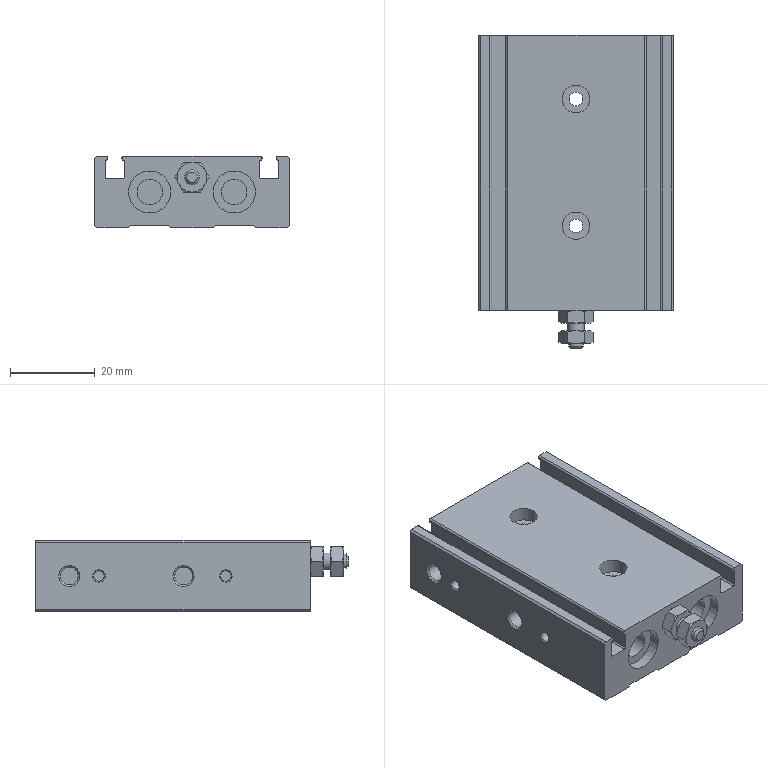Part | STEP file | ROTATION MC_NEW VER-0610_475 | 1 solid | 141 faces | box 46 x 74 x 17 mm | volume 39831 mm3 | plane 66 | cylinder 40 | cone 35 | commonest cylinder face diameters 0.8 x12 10 x6 0.4 x4 2.459 x4 4.134 x4 3.242 x2